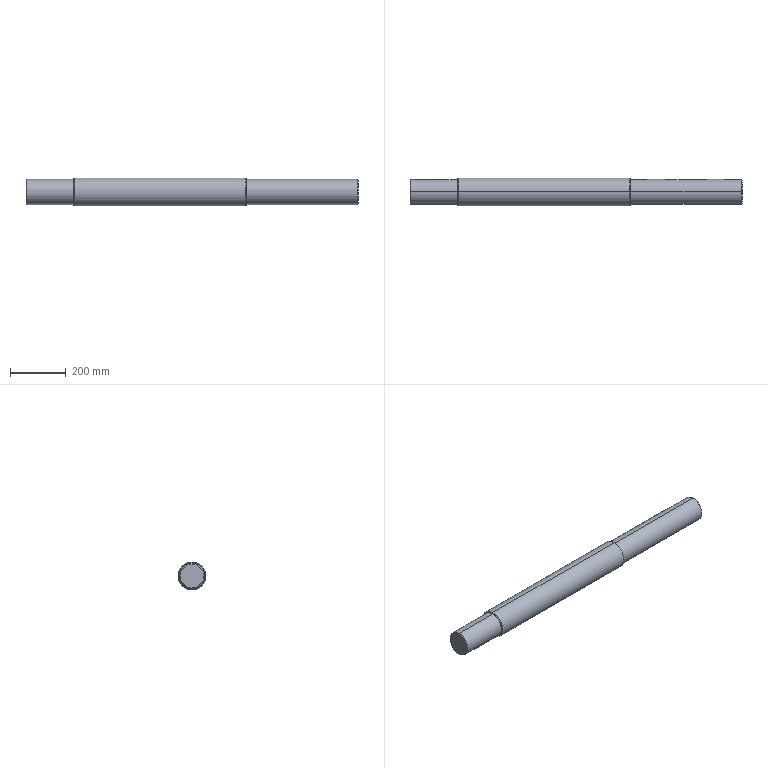Part | STEP file | 01-Main drive shaft | 1 solid | 32 faces | box 1190 x 100 x 100 mm | volume 8433276 mm3 | cylinder 10 | plane 10 | cone 8 | torus 4 | commonest cylinder face diameters 25 x4 90 x4 100 x2